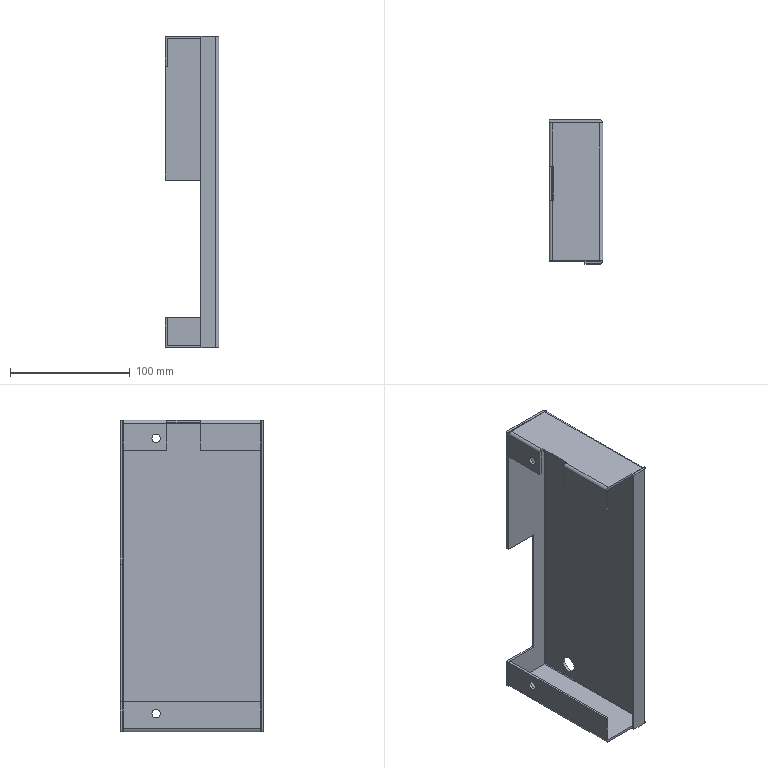Part | STEP file | Left Cover Plate | 1 solid | 62 faces | box 45 x 120 x 260 mm | volume 111585 mm3 | plane 40 | cylinder 22 | commonest cylinder face diameters 1 x7 5 x7 7 x4 13 x4